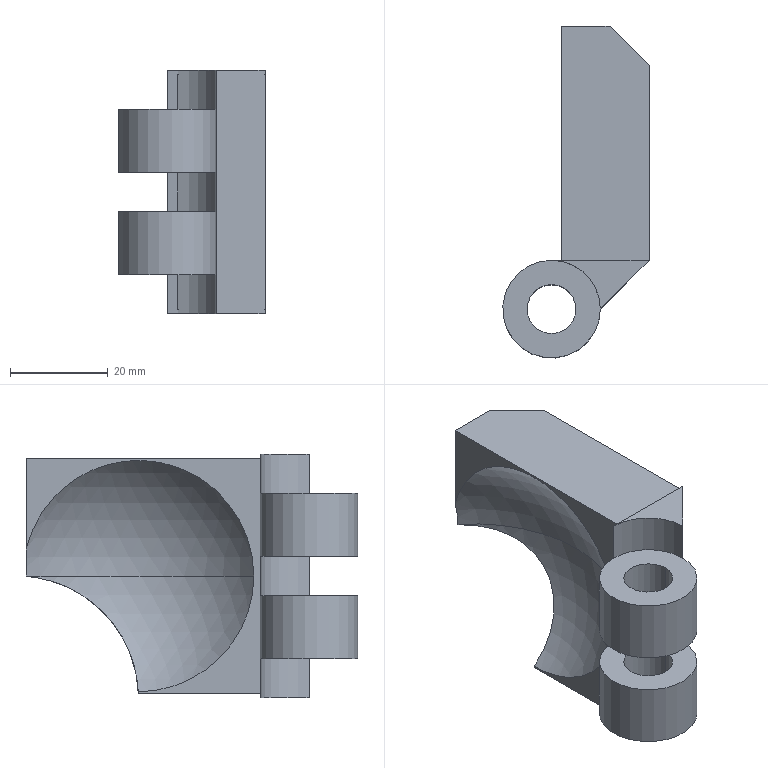Part | SolidWorks | features BaseBody 1 | 1 solid | 26 faces | box 30 x 68 x 50 mm | volume 32922 mm3 | plane 14 | cylinder 10 | sphere 2 | commonest cylinder face diameters 20 x5 10 x4 50 x1
STEP:
#1=CARTESIAN_POINT('',(-5.,0.,21.));
#2=VERTEX_POINT('',#1);
#3=CARTESIAN_POINT('',(5.,0.,21.));
#4=VERTEX_POINT('',#3);
#5=CARTESIAN_POINT('',(0.,0.,21.));
#6=DIRECTION('',(0.,0.,1.));
#7=DIRECTION('',(-1.,0.,0.));
#8=AXIS2_PLACEMENT_3D('',#5,#6,#7);
#9=CIRCLE('',#8,5.);
#10=EDGE_CURVE('',#2,#4,#9,.T.);
#11=ORIENTED_EDGE('',*,*,#10,.T.);
#12=CARTESIAN_POINT('',(5.,0.,8.));
#13=VERTEX_POINT('',#12);
#14=CARTESIAN_POINT('',(5.,0.,0.));
#15=DIRECTION('',(0.,0.,-1.));
#16=VECTOR('',#15,1000.);
#17=LINE('',#14,#16);
#18=EDGE_CURVE('',#4,#13,#17,.T.);
#19=ORIENTED_EDGE('',*,*,#18,.T.);
#20=CARTESIAN_POINT('',(-5.,0.,8.));
#21=VERTEX_POINT('',#20);
#22=CARTESIAN_POINT('',(0.,0.,8.));
#23=DIRECTION('',(0.,0.,-1.));
#24=DIRECTION('',(-1.,0.,0.));
#25=AXIS2_PLACEMENT_3D('',#22,#23,#24);
#26=CIRCLE('',#25,5.);
#27=EDGE_CURVE('',#13,#21,#26,.T.);
#28=ORIENTED_EDGE('',*,*,#27,.T.);
#29=CARTESIAN_POINT('',(-5.,0.,0.));
#30=DIRECTION('',(0.,0.,-1.));
#31=VECTOR('',#30,1000.);
#32=LINE('',#29,#31);
#33=EDGE_CURVE('',#2,#21,#32,.T.);
#34=ORIENTED_EDGE('',*,*,#33,.F.);
#35=EDGE_LOOP('',(#11,#19,#28,#34));
#36=FACE_OUTER_BOUND('',#35,.T.);
#37=CARTESIAN_POINT('',(0.,0.,0.));
#38=DIRECTION('',(0.,0.,-1.));
#39=DIRECTION('',(-1.,0.,0.));
#40=AXIS2_PLACEMENT_3D('',#37,#38,#39);
#41=CYLINDRICAL_SURFACE('',#40,5.);
#42=ADVANCED_FACE('',(#36),#41,.F.);
#43=CARTESIAN_POINT('',(2.,35.036,1.342));
#44=VERTEX_POINT('',#43);
#45=CARTESIAN_POINT('',(2.,11.342,25.));
#46=VERTEX_POINT('',#45);
#47=CARTESIAN_POINT('',(2.,35.,25.));
#48=DIRECTION('',(-1.,0.,0.));
#49=DIRECTION('',(0.,0.,1.));
#50=AXIS2_PLACEMENT_3D('',#47,#48,#49);
#51=CIRCLE('',#50,23.658);
#52=EDGE_CURVE('',#44,#46,#51,.T.);
#53=ORIENTED_EDGE('',*,*,#52,.T.);
#54=CARTESIAN_POINT('',(2.865,58.,25.));
#55=VERTEX_POINT('',#54);
#56=CARTESIAN_POINT('',(-15.321,35.,25.));
#57=DIRECTION('',(0.,0.,1.));
#58=DIRECTION('',(1.,0.,0.));
#59=AXIS2_PLACEMENT_3D('',#56,#57,#58);
#60=CIRCLE('',#59,29.321);
#61=EDGE_CURVE('',#46,#55,#60,.T.);
#62=ORIENTED_EDGE('',*,*,#61,.T.);
#63=CARTESIAN_POINT('',(2.865,58.,24.92));
#64=VERTEX_POINT('',#63);
#65=CARTESIAN_POINT('',(-15.321,58.,25.));
#66=DIRECTION('',(0.,1.,0.));
#67=DIRECTION('',(0.,0.,1.));
#68=AXIS2_PLACEMENT_3D('',#65,#66,#67);
#69=CIRCLE('',#68,18.186);
#70=EDGE_CURVE('',#55,#64,#69,.T.);
#71=ORIENTED_EDGE('',*,*,#70,.T.);
#72=CARTESIAN_POINT('',(2.865,58.,24.92));
#73=CARTESIAN_POINT('',(4.253,56.902,24.832));
#74=CARTESIAN_POINT('',(5.518,55.699,24.663));
#75=CARTESIAN_POINT('',(6.944,54.07,24.289));
#76=CARTESIAN_POINT('',(7.221,53.738,24.206));
#77=CARTESIAN_POINT('',(7.76,53.062,24.021));
#78=CARTESIAN_POINT('',(8.021,52.717,23.918));
#79=CARTESIAN_POINT('',(8.769,51.678,23.586));
#80=CARTESIAN_POINT('',(9.224,50.976,23.327));
#81=CARTESIAN_POINT('',(10.044,49.559,22.728));
#82=CARTESIAN_POINT('',(10.409,48.843,22.387));
#83=CARTESIAN_POINT('',(10.887,47.761,21.803));
#84=CARTESIAN_POINT('',(11.035,47.398,21.596));
#85=CARTESIAN_POINT('',(11.304,46.674,21.156));
#86=CARTESIAN_POINT('',(11.424,46.316,20.927));
#87=CARTESIAN_POINT('',(11.74,45.258,20.209));
#88=CARTESIAN_POINT('',(11.894,44.572,19.691));
#89=CARTESIAN_POINT('',(12.039,43.575,18.852));
#90=CARTESIAN_POINT('',(12.073,43.248,18.562));
#91=CARTESIAN_POINT('',(12.111,42.604,17.96));
#92=CARTESIAN_POINT('',(12.116,42.286,17.647));
#93=CARTESIAN_POINT('',(12.082,41.364,16.688));
#94=CARTESIAN_POINT('',(11.999,40.792,16.025));
#95=CARTESIAN_POINT('',(11.789,39.994,14.998));
#96=CARTESIAN_POINT('',(11.704,39.738,14.65));
#97=CARTESIAN_POINT('',(11.506,39.246,13.944));
#98=CARTESIAN_POINT('',(11.391,39.008,13.584));
#99=CARTESIAN_POINT('',(11.008,38.334,12.502));
#100=CARTESIAN_POINT('',(10.7,37.935,11.78));
#101=CARTESIAN_POINT('',(10.166,37.401,10.697));
#102=CARTESIAN_POINT('',(9.975,37.234,10.336));
#103=CARTESIAN_POINT('',(9.57,36.92,9.616));
#104=CARTESIAN_POINT('',(9.354,36.773,9.255));
#105=CARTESIAN_POINT('',(8.225,36.094,7.472));
#106=CARTESIAN_POINT('',(7.167,35.724,6.114));
#107=CARTESIAN_POINT('',(4.755,35.22,3.557));
#108=CARTESIAN_POINT('',(3.432,35.092,2.39));
#109=CARTESIAN_POINT('',(2.,35.036,1.342));
#110=B_SPLINE_CURVE_WITH_KNOTS('',3,(#72,#73,#74,#75,#76,#77,#78,#79,#80,#81,#82,#83,#84,#85,#86,#87,#88,#89,#90,#91,#92,#93,#94,#95,#96,#97,#98,#99,#100,#101,#102,#103,#104,#105,#106,#107,#108,#109),.UNSPECIFIED.,.F.,.F.,(4,2,2,2,2,2,2,2,2,2,2,2,2,2,2,2,2,2,4),(0.,0.005258,0.006573,0.007887,0.01052,0.01315,0.01446,0.01577,0.0184,0.01972,0.02103,0.02366,0.02498,0.02629,0.02892,0.03023,0.03155,0.03681,0.04206),.UNSPECIFIED.);
#111=EDGE_CURVE('',#64,#44,#110,.T.);
#112=ORIENTED_EDGE('',*,*,#111,.T.);
#113=EDGE_LOOP('',(#53,#62,#71,#112));
#114=FACE_OUTER_BOUND('',#113,.T.);
#115=CARTESIAN_POINT('',(-15.321,35.,25.));
#116=DIRECTION('',(0.,0.,-1.));
#117=DIRECTION('',(1.,0.,0.));
#118=AXIS2_PLACEMENT_3D('',#115,#116,#117);
#119=SPHERICAL_SURFACE('',#118,29.321);
#120=ADVANCED_FACE('',(#114),#119,.F.);
#121=CARTESIAN_POINT('',(-5.,0.,42.));
#122=VERTEX_POINT('',#121);
#123=CARTESIAN_POINT('',(5.,0.,42.));
#124=VERTEX_POINT('',#123);
#125=CARTESIAN_POINT('',(0.,0.,42.));
#126=DIRECTION('',(0.,0.,1.));
#127=DIRECTION('',(-1.,0.,0.));
#128=AXIS2_PLACEMENT_3D('',#125,#126,#127);
#129=CIRCLE('',#128,5.);
#130=EDGE_CURVE('',#122,#124,#129,.T.);
#131=ORIENTED_EDGE('',*,*,#130,.T.);
#132=CARTESIAN_POINT('',(5.,0.,29.));
#133=VERTEX_POINT('',#132);
#134=CARTESIAN_POINT('',(5.,0.,0.));
#135=DIRECTION('',(0.,0.,-1.));
#136=VECTOR('',#135,1000.);
#137=LINE('',#134,#136);
#138=EDGE_CURVE('',#124,#133,#137,.T.);
#139=ORIENTED_EDGE('',*,*,#138,.T.);
#140=CARTESIAN_POINT('',(-5.,0.,29.));
#141=VERTEX_POINT('',#140);
#142=CARTESIAN_POINT('',(0.,0.,29.));
#143=DIRECTION('',(0.,0.,-1.));
#144=DIRECTION('',(-1.,0.,0.));
#145=AXIS2_PLACEMENT_3D('',#142,#143,#144);
#146=CIRCLE('',#145,5.);
#147=EDGE_CURVE('',#133,#141,#146,.T.);
#148=ORIENTED_EDGE('',*,*,#147,.T.);
#149=CARTESIAN_POINT('',(-5.,0.,0.));
#150=DIRECTION('',(0.,0.,-1.));
#151=VECTOR('',#150,1000.);
#152=LINE('',#149,#151);
#153=EDGE_CURVE('',#122,#141,#152,.T.);
#154=ORIENTED_EDGE('',*,*,#153,.F.);
#155=EDGE_LOOP('',(#131,#139,#148,#154));
#156=FACE_OUTER_BOUND('',#155,.T.);
#157=CARTESIAN_POINT('',(0.,0.,0.));
#158=DIRECTION('',(0.,0.,-1.));
#159=DIRECTION('',(-1.,0.,0.));
#160=AXIS2_PLACEMENT_3D('',#157,#158,#159);
#161=CYLINDRICAL_SURFACE('',#160,5.);
#162=ADVANCED_FACE('',(#156),#161,.F.);
#163=CARTESIAN_POINT('',(0.,0.,29.));
#164=DIRECTION('',(0.,0.,-1.));
#165=DIRECTION('',(-1.,0.,0.));
#166=AXIS2_PLACEMENT_3D('',#163,#164,#165);
#167=CIRCLE('',#166,5.);
#168=EDGE_CURVE('',#141,#133,#167,.T.);
#169=ORIENTED_EDGE('',*,*,#168,.F.);
#170=ORIENTED_EDGE('',*,*,#147,.F.);
#171=EDGE_LOOP('',(#169,#170));
#172=FACE_BOUND('',#171,.T.);
#173=CARTESIAN_POINT('',(0.,10.,29.));
#174=VERTEX_POINT('',#173);
#175=CARTESIAN_POINT('',(10.,0.,29.));
#176=VERTEX_POINT('',#175);
#177=CARTESIAN_POINT('',(0.,0.,29.));
#178=DIRECTION('',(0.,0.,1.));
#179=DIRECTION('',(0.,1.,0.));
#180=AXIS2_PLACEMENT_3D('',#177,#178,#179);
#181=CIRCLE('',#180,10.);
#182=EDGE_CURVE('',#174,#176,#181,.T.);
#183=ORIENTED_EDGE('',*,*,#182,.F.);
#184=CARTESIAN_POINT('',(0.,0.,29.));
#185=DIRECTION('',(0.,0.,-1.));
#186=DIRECTION('',(1.,0.,0.));
#187=AXIS2_PLACEMENT_3D('',#184,#185,#186);
#188=CIRCLE('',#187,10.);
#189=EDGE_CURVE('',#174,#176,#188,.T.);
#190=ORIENTED_EDGE('',*,*,#189,.T.);
#191=EDGE_LOOP('',(#183,#190));
#192=FACE_OUTER_BOUND('',#191,.T.);
#193=CARTESIAN_POINT('',(-10.,0.,29.));
#194=DIRECTION('',(0.,0.,1.));
#195=DIRECTION('',(1.,0.,0.));
#196=AXIS2_PLACEMENT_3D('',#193,#194,#195);
#197=PLANE('',#196);
#198=ADVANCED_FACE('',(#172,#192),#197,.F.);
#199=CARTESIAN_POINT('',(10.,0.,21.));
#200=VERTEX_POINT('',#199);
#201=CARTESIAN_POINT('',(10.,0.,0.));
#202=DIRECTION('',(0.,0.,1.));
#203=VECTOR('',#202,1000.);
#204=LINE('',#201,#203);
#205=EDGE_CURVE('',#200,#176,#204,.T.);
#206=ORIENTED_EDGE('',*,*,#205,.T.);
#207=ORIENTED_EDGE('',*,*,#189,.F.);
#208=CARTESIAN_POINT('',(0.,10.,21.));
#209=VERTEX_POINT('',#208);
#210=CARTESIAN_POINT('',(0.,10.,0.));
#211=DIRECTION('',(0.,0.,1.));
#212=VECTOR('',#211,1000.);
#213=LINE('',#210,#212);
#214=EDGE_CURVE('',#209,#174,#213,.T.);
#215=ORIENTED_EDGE('',*,*,#214,.F.);
#216=CARTESIAN_POINT('',(0.,0.,21.));
#217=DIRECTION('',(0.,0.,-1.));
#218=DIRECTION('',(1.,0.,0.));
#219=AXIS2_PLACEMENT_3D('',#216,#217,#218);
#220=CIRCLE('',#219,10.);
#221=EDGE_CURVE('',#209,#200,#220,.T.);
#222=ORIENTED_EDGE('',*,*,#221,.T.);
#223=EDGE_LOOP('',(#206,#207,#215,#222));
#224=FACE_OUTER_BOUND('',#223,.T.);
#225=CARTESIAN_POINT('',(0.,0.,25.));
#226=DIRECTION('',(0.,0.,1.));
#227=DIRECTION('',(-1.,0.,0.));
#228=AXIS2_PLACEMENT_3D('',#225,#226,#227);
#229=CYLINDRICAL_SURFACE('',#228,10.);
#230=ADVANCED_FACE('',(#224),#229,.F.);
#231=ORIENTED_EDGE('',*,*,#10,.F.);
#232=CARTESIAN_POINT('',(0.,0.,21.));
#233=DIRECTION('',(0.,0.,1.));
#234=DIRECTION('',(-1.,0.,0.));
#235=AXIS2_PLACEMENT_3D('',#232,#233,#234);
#236=CIRCLE('',#235,5.);
#237=EDGE_CURVE('',#4,#2,#236,.T.);
#238=ORIENTED_EDGE('',*,*,#237,.F.);
#239=EDGE_LOOP('',(#231,#238));
#240=FACE_BOUND('',#239,.T.);
#241=CARTESIAN_POINT('',(0.,0.,21.));
#242=DIRECTION('',(0.,0.,-1.));
#243=DIRECTION('',(0.,1.,0.));
#244=AXIS2_PLACEMENT_3D('',#241,#242,#243);
#245=CIRCLE('',#244,10.);
#246=EDGE_CURVE('',#200,#209,#245,.T.);
#247=ORIENTED_EDGE('',*,*,#246,.F.);
#248=ORIENTED_EDGE('',*,*,#221,.F.);
#249=EDGE_LOOP('',(#247,#248));
#250=FACE_OUTER_BOUND('',#249,.T.);
#251=CARTESIAN_POINT('',(0.,0.,21.));
#252=DIRECTION('',(0.,0.,-1.));
#253=DIRECTION('',(0.,-1.,0.));
#254=AXIS2_PLACEMENT_3D('',#251,#252,#253);
#255=PLANE('',#254);
#256=ADVANCED_FACE('',(#240,#250),#255,.F.);
#257=CARTESIAN_POINT('',(0.,0.,8.));
#258=DIRECTION('',(0.,0.,-1.));
#259=DIRECTION('',(-1.,0.,0.));
#260=AXIS2_PLACEMENT_3D('',#257,#258,#259);
#261=CIRCLE('',#260,5.);
#262=EDGE_CURVE('',#21,#13,#261,.T.);
#263=ORIENTED_EDGE('',*,*,#262,.F.);
#264=ORIENTED_EDGE('',*,*,#27,.F.);
#265=EDGE_LOOP('',(#263,#264));
#266=FACE_BOUND('',#265,.T.);
#267=CARTESIAN_POINT('',(0.,10.,8.));
#268=VERTEX_POINT('',#267);
#269=CARTESIAN_POINT('',(10.,0.,8.));
#270=VERTEX_POINT('',#269);
#271=CARTESIAN_POINT('',(0.,0.,8.));
#272=DIRECTION('',(0.,0.,1.));
#273=DIRECTION('',(0.,1.,0.));
#274=AXIS2_PLACEMENT_3D('',#271,#272,#273);
#275=CIRCLE('',#274,10.);
#276=EDGE_CURVE('',#268,#270,#275,.T.);
#277=ORIENTED_EDGE('',*,*,#276,.F.);
#278=CARTESIAN_POINT('',(0.,0.,8.));
#279=DIRECTION('',(0.,0.,-1.));
#280=DIRECTION('',(1.,0.,0.));
#281=AXIS2_PLACEMENT_3D('',#278,#279,#280);
#282=CIRCLE('',#281,10.);
#283=EDGE_CURVE('',#268,#270,#282,.T.);
#284=ORIENTED_EDGE('',*,*,#283,.T.);
#285=EDGE_LOOP('',(#277,#284));
#286=FACE_OUTER_BOUND('',#285,.T.);
#287=CARTESIAN_POINT('',(-10.,0.,8.));
#288=DIRECTION('',(0.,0.,1.));
#289=DIRECTION('',(1.,0.,0.));
#290=AXIS2_PLACEMENT_3D('',#287,#288,#289);
#291=PLANE('',#290);
#292=ADVANCED_FACE('',(#266,#286),#291,.F.);
#293=CARTESIAN_POINT('',(10.,0.,0.));
#294=VERTEX_POINT('',#293);
#295=CARTESIAN_POINT('',(10.,0.,0.));
#296=DIRECTION('',(0.,0.,1.));
#297=VECTOR('',#296,1000.);
#298=LINE('',#295,#297);
#299=EDGE_CURVE('',#294,#270,#298,.T.);
#300=ORIENTED_EDGE('',*,*,#299,.T.);
#301=ORIENTED_EDGE('',*,*,#283,.F.);
#302=CARTESIAN_POINT('',(0.,10.,0.));
#303=VERTEX_POINT('',#302);
#304=CARTESIAN_POINT('',(0.,10.,0.));
#305=DIRECTION('',(0.,0.,1.));
#306=VECTOR('',#305,1000.);
#307=LINE('',#304,#306);
#308=EDGE_CURVE('',#303,#268,#307,.T.);
#309=ORIENTED_EDGE('',*,*,#308,.F.);
#310=CARTESIAN_POINT('',(0.,0.,0.));
#311=DIRECTION('',(0.,0.,1.));
#312=DIRECTION('',(-1.,0.,0.));
#313=AXIS2_PLACEMENT_3D('',#310,#311,#312);
#314=CIRCLE('',#313,10.);
#315=EDGE_CURVE('',#294,#303,#314,.T.);
#316=ORIENTED_EDGE('',*,*,#315,.F.);
#317=EDGE_LOOP('',(#300,#301,#309,#316));
#318=FACE_OUTER_BOUND('',#317,.T.);
#319=CARTESIAN_POINT('',(0.,0.,4.));
#320=DIRECTION('',(0.,0.,1.));
#321=DIRECTION('',(-1.,0.,0.));
#322=AXIS2_PLACEMENT_3D('',#319,#320,#321);
#323=CYLINDRICAL_SURFACE('',#322,10.);
#324=ADVANCED_FACE('',(#318),#323,.F.);
#325=CARTESIAN_POINT('',(10.,0.,42.));
#326=VERTEX_POINT('',#325);
#327=CARTESIAN_POINT('',(10.,0.,50.));
#328=VERTEX_POINT('',#327);
#329=CARTESIAN_POINT('',(10.,0.,0.));
#330=DIRECTION('',(0.,0.,1.));
#331=VECTOR('',#330,1000.);
#332=LINE('',#329,#331);
#333=EDGE_CURVE('',#326,#328,#332,.T.);
#334=ORIENTED_EDGE('',*,*,#333,.T.);
#335=CARTESIAN_POINT('',(0.,10.,50.));
#336=VERTEX_POINT('',#335);
#337=CARTESIAN_POINT('',(0.,0.,50.));
#338=DIRECTION('',(0.,0.,-1.));
#339=DIRECTION('',(-1.,0.,0.));
#340=AXIS2_PLACEMENT_3D('',#337,#338,#339);
#341=CIRCLE('',#340,10.);
#342=EDGE_CURVE('',#336,#328,#341,.T.);
#343=ORIENTED_EDGE('',*,*,#342,.F.);
#344=CARTESIAN_POINT('',(0.,10.,42.));
#345=VERTEX_POINT('',#344);
#346=CARTESIAN_POINT('',(0.,10.,0.));
#347=DIRECTION('',(0.,0.,1.));
#348=VECTOR('',#347,1000.);
#349=LINE('',#346,#348);
#350=EDGE_CURVE('',#345,#336,#349,.T.);
#351=ORIENTED_EDGE('',*,*,#350,.F.);
#352=CARTESIAN_POINT('',(0.,0.,42.));
#353=DIRECTION('',(0.,0.,-1.));
#354=DIRECTION('',(1.,0.,0.));
#355=AXIS2_PLACEMENT_3D('',#352,#353,#354);
#356=CIRCLE('',#355,10.);
#357=EDGE_CURVE('',#345,#326,#356,.T.);
#358=ORIENTED_EDGE('',*,*,#357,.T.);
#359=EDGE_LOOP('',(#334,#343,#351,#358));
#360=FACE_OUTER_BOUND('',#359,.T.);
#361=CARTESIAN_POINT('',(0.,0.,46.));
#362=DIRECTION('',(0.,0.,1.));
#363=DIRECTION('',(-1.,0.,0.));
#364=AXIS2_PLACEMENT_3D('',#361,#362,#363);
#365=CYLINDRICAL_SURFACE('',#364,10.);
#366=ADVANCED_FACE('',(#360),#365,.F.);
#367=ORIENTED_EDGE('',*,*,#130,.F.);
#368=CARTESIAN_POINT('',(0.,0.,42.));
#369=DIRECTION('',(0.,0.,1.));
#370=DIRECTION('',(-1.,0.,0.));
#371=AXIS2_PLACEMENT_3D('',#368,#369,#370);
#372=CIRCLE('',#371,5.);
#373=EDGE_CURVE('',#124,#122,#372,.T.);
#374=ORIENTED_EDGE('',*,*,#373,.F.);
#375=EDGE_LOOP('',(#367,#374));
#376=FACE_BOUND('',#375,.T.);
#377=CARTESIAN_POINT('',(0.,0.,42.));
#378=DIRECTION('',(0.,0.,-1.));
#379=DIRECTION('',(0.,1.,0.));
#380=AXIS2_PLACEMENT_3D('',#377,#378,#379);
#381=CIRCLE('',#380,10.);
#382=EDGE_CURVE('',#326,#345,#381,.T.);
#383=ORIENTED_EDGE('',*,*,#382,.F.);
#384=ORIENTED_EDGE('',*,*,#357,.F.);
#385=EDGE_LOOP('',(#383,#384));
#386=FACE_OUTER_BOUND('',#385,.T.);
#387=CARTESIAN_POINT('',(0.,0.,42.));
#388=DIRECTION('',(0.,0.,-1.));
#389=DIRECTION('',(0.,-1.,0.));
#390=AXIS2_PLACEMENT_3D('',#387,#388,#389);
#391=PLANE('',#390);
#392=ADVANCED_FACE('',(#376,#386),#391,.F.);
#393=ORIENTED_EDGE('',*,*,#315,.T.);
#394=CARTESIAN_POINT('',(20.,10.,0.));
#395=VERTEX_POINT('',#394);
#396=CARTESIAN_POINT('',(7.926,10.,0.));
#397=DIRECTION('',(1.,0.,0.));
#398=VECTOR('',#397,1000.);
#399=LINE('',#396,#398);
#400=EDGE_CURVE('',#303,#395,#399,.T.);
#401=ORIENTED_EDGE('',*,*,#400,.T.);
#402=CARTESIAN_POINT('',(10.,0.,0.));
#403=DIRECTION('',(0.7071,0.7071,0.));
#404=VECTOR('',#403,1000.);
#405=LINE('',#402,#404);
#406=EDGE_CURVE('',#294,#395,#405,.T.);
#407=ORIENTED_EDGE('',*,*,#406,.F.);
#408=EDGE_LOOP('',(#393,#401,#407));
#409=FACE_OUTER_BOUND('',#408,.T.);
#410=CARTESIAN_POINT('',(4.852,2.817,0.));
#411=DIRECTION('',(0.,0.,1.));
#412=DIRECTION('',(1.,0.,0.));
#413=AXIS2_PLACEMENT_3D('',#410,#411,#412);
#414=PLANE('',#413);
#415=ADVANCED_FACE('',(#409),#414,.F.);
#416=ORIENTED_EDGE('',*,*,#182,.T.);
#417=CARTESIAN_POINT('',(10.,0.,0.));
#418=DIRECTION('',(0.,0.,1.));
#419=VECTOR('',#418,1000.);
#420=LINE('',#417,#419);
#421=EDGE_CURVE('',#176,#326,#420,.T.);
#422=ORIENTED_EDGE('',*,*,#421,.T.);
#423=ORIENTED_EDGE('',*,*,#382,.T.);
#424=CARTESIAN_POINT('',(0.,10.,0.));
#425=DIRECTION('',(0.,0.,1.));
#426=VECTOR('',#425,1000.);
#427=LINE('',#424,#426);
#428=EDGE_CURVE('',#174,#345,#427,.T.);
#429=ORIENTED_EDGE('',*,*,#428,.F.);
#430=EDGE_LOOP('',(#416,#422,#423,#429));
#431=FACE_OUTER_BOUND('',#430,.T.);
#432=CARTESIAN_POINT('',(0.,0.,0.));
#433=DIRECTION('',(0.,0.,-1.));
#434=DIRECTION('',(0.,1.,0.));
#435=AXIS2_PLACEMENT_3D('',#432,#433,#434);
#436=CYLINDRICAL_SURFACE('',#435,10.);
#437=ADVANCED_FACE('',(#431),#436,.T.);
#438=ORIENTED_EDGE('',*,*,#246,.T.);
#439=CARTESIAN_POINT('',(0.,10.,0.));
#440=DIRECTION('',(0.,0.,1.));
#441=VECTOR('',#440,1000.);
#442=LINE('',#439,#441);
#443=EDGE_CURVE('',#268,#209,#442,.T.);
#444=ORIENTED_EDGE('',*,*,#443,.F.);
#445=ORIENTED_EDGE('',*,*,#276,.T.);
#446=CARTESIAN_POINT('',(10.,0.,0.));
#447=DIRECTION('',(0.,0.,1.));
#448=VECTOR('',#447,1000.);
#449=LINE('',#446,#448);
#450=EDGE_CURVE('',#270,#200,#449,.T.);
#451=ORIENTED_EDGE('',*,*,#450,.T.);
#452=EDGE_LOOP('',(#438,#444,#445,#451));
#453=FACE_OUTER_BOUND('',#452,.T.);
#454=CARTESIAN_POINT('',(0.,0.,0.));
#455=DIRECTION('',(0.,0.,-1.));
#456=DIRECTION('',(0.,1.,0.));
#457=AXIS2_PLACEMENT_3D('',#454,#455,#456);
#458=CYLINDRICAL_SURFACE('',#457,10.);
#459=ADVANCED_FACE('',(#453),#458,.T.);
#460=ORIENTED_EDGE('',*,*,#111,.F.);
#461=CARTESIAN_POINT('',(12.,58.,24.92));
#462=VERTEX_POINT('',#461);
#463=CARTESIAN_POINT('',(2.,58.,24.92));
#464=DIRECTION('',(-1.,0.,0.));
#465=VECTOR('',#464,1000.);
#466=LINE('',#463,#465);
#467=EDGE_CURVE('',#462,#64,#466,.T.);
#468=ORIENTED_EDGE('',*,*,#467,.F.);
#469=CARTESIAN_POINT('',(20.,50.,22.913));
#470=VERTEX_POINT('',#469);
#471=CARTESIAN_POINT('',(20.,50.,22.913));
#472=CARTESIAN_POINT('',(17.457,52.543,24.023));
#473=CARTESIAN_POINT('',(14.766,55.234,24.698));
#474=CARTESIAN_POINT('',(12.,58.,24.92));
#475=(BOUNDED_CURVE()B_SPLINE_CURVE(3,(#471,#472,#473,#474),.UNSPECIFIED.,.F.,.F.)B_SPLINE_CURVE_WITH_KNOTS((4,4),(4.301,4.632),.UNSPECIFIED.)CURVE()GEOMETRIC_REPRESENTATION_ITEM()RATIONAL_B_SPLINE_CURVE((1.,0.9909,0.9909,1.))REPRESENTATION_ITEM(''));
#476=EDGE_CURVE('',#470,#462,#475,.T.);
#477=ORIENTED_EDGE('',*,*,#476,.F.);
#478=CARTESIAN_POINT('',(20.,35.02,1.));
#479=VERTEX_POINT('',#478);
#480=CARTESIAN_POINT('',(20.,60.,0.));
#481=DIRECTION('',(-1.,0.,0.));
#482=DIRECTION('',(0.,0.,-1.));
#483=AXIS2_PLACEMENT_3D('',#480,#481,#482);
#484=CIRCLE('',#483,25.);
#485=EDGE_CURVE('',#479,#470,#484,.T.);
#486=ORIENTED_EDGE('',*,*,#485,.F.);
#487=CARTESIAN_POINT('',(2.,35.02,1.));
#488=VERTEX_POINT('',#487);
#489=CARTESIAN_POINT('',(2.,35.02,1.));
#490=DIRECTION('',(1.,0.,0.));
#491=VECTOR('',#490,1000.);
#492=LINE('',#489,#491);
#493=EDGE_CURVE('',#488,#479,#492,.T.);
#494=ORIENTED_EDGE('',*,*,#493,.F.);
#495=CARTESIAN_POINT('',(2.,60.,0.));
#496=DIRECTION('',(1.,0.,0.));
#497=DIRECTION('',(0.,0.,-1.));
#498=AXIS2_PLACEMENT_3D('',#495,#496,#497);
#499=CIRCLE('',#498,25.);
#500=EDGE_CURVE('',#44,#488,#499,.T.);
#501=ORIENTED_EDGE('',*,*,#500,.F.);
#502=EDGE_LOOP('',(#460,#468,#477,#486,#494,#501));
#503=FACE_OUTER_BOUND('',#502,.T.);
#504=CARTESIAN_POINT('',(2.,60.,0.));
#505=DIRECTION('',(-1.,0.,0.));
#506=DIRECTION('',(0.,0.,-1.));
#507=AXIS2_PLACEMENT_3D('',#504,#505,#506);
#508=CYLINDRICAL_SURFACE('',#507,25.);
#509=ADVANCED_FACE('',(#503),#508,.F.);
#510=ORIENTED_EDGE('',*,*,#467,.T.);
#511=ORIENTED_EDGE('',*,*,#70,.F.);
#512=CARTESIAN_POINT('',(2.,58.,30.542));
#513=VERTEX_POINT('',#512);
#514=CARTESIAN_POINT('',(-15.321,58.,25.));
#515=DIRECTION('',(0.,1.,0.));
#516=DIRECTION('',(0.,0.,1.));
#517=AXIS2_PLACEMENT_3D('',#514,#515,#516);
#518=CIRCLE('',#517,18.186);
#519=EDGE_CURVE('',#513,#55,#518,.T.);
#520=ORIENTED_EDGE('',*,*,#519,.F.);
#521=CARTESIAN_POINT('',(2.,58.,49.));
#522=VERTEX_POINT('',#521);
#523=CARTESIAN_POINT('',(2.,58.,50.));
#524=DIRECTION('',(0.,0.,-1.));
#525=VECTOR('',#524,1000.);
#526=LINE('',#523,#525);
#527=EDGE_CURVE('',#522,#513,#526,.T.);
#528=ORIENTED_EDGE('',*,*,#527,.F.);
#529=CARTESIAN_POINT('',(12.,58.,49.));
#530=VERTEX_POINT('',#529);
#531=CARTESIAN_POINT('',(7.,58.,49.));
#532=DIRECTION('',(1.,0.,0.));
#533=VECTOR('',#532,1000.);
#534=LINE('',#531,#533);
#535=EDGE_CURVE('',#522,#530,#534,.T.);
#536=ORIENTED_EDGE('',*,*,#535,.T.);
#537=CARTESIAN_POINT('',(12.,58.,25.));
#538=DIRECTION('',(0.,0.,1.));
#539=VECTOR('',#538,1000.);
#540=LINE('',#537,#539);
#541=EDGE_CURVE('',#462,#530,#540,.T.);
#542=ORIENTED_EDGE('',*,*,#541,.F.);
#543=EDGE_LOOP('',(#510,#511,#520,#528,#536,#542));
#544=FACE_OUTER_BOUND('',#543,.T.);
#545=CARTESIAN_POINT('',(12.,58.,50.));
#546=DIRECTION('',(0.,-1.,0.));
#547=DIRECTION('',(0.,0.,-1.));
#548=AXIS2_PLACEMENT_3D('',#545,#546,#547);
#549=PLANE('',#548);
#550=ADVANCED_FACE('',(#544),#549,.F.);
#551=ORIENTED_EDGE('',*,*,#500,.T.);
#552=CARTESIAN_POINT('',(2.,10.,1.));
#553=VERTEX_POINT('',#552);
#554=CARTESIAN_POINT('',(2.,59.,1.));
#555=DIRECTION('',(0.,-1.,0.));
#556=VECTOR('',#555,1000.);
#557=LINE('',#554,#556);
#558=EDGE_CURVE('',#488,#553,#557,.T.);
#559=ORIENTED_EDGE('',*,*,#558,.T.);
#560=CARTESIAN_POINT('',(2.,10.,49.));
#561=VERTEX_POINT('',#560);
#562=CARTESIAN_POINT('',(2.,10.,50.));
#563=DIRECTION('',(0.,0.,-1.));
#564=VECTOR('',#563,1000.);
#565=LINE('',#562,#564);
#566=EDGE_CURVE('',#561,#553,#565,.T.);
#567=ORIENTED_EDGE('',*,*,#566,.F.);
#568=CARTESIAN_POINT('',(2.,59.,49.));
#569=DIRECTION('',(0.,1.,0.));
#570=VECTOR('',#569,1000.);
#571=LINE('',#568,#570);
#572=EDGE_CURVE('',#561,#522,#571,.T.);
#573=ORIENTED_EDGE('',*,*,#572,.T.);
#574=ORIENTED_EDGE('',*,*,#527,.T.);
#575=CARTESIAN_POINT('',(2.,35.,25.));
#576=DIRECTION('',(-1.,0.,0.));
#577=DIRECTION('',(0.,0.,1.));
#578=AXIS2_PLACEMENT_3D('',#575,#576,#577);
#579=CIRCLE('',#578,23.658);
#580=EDGE_CURVE('',#46,#513,#579,.T.);
#581=ORIENTED_EDGE('',*,*,#580,.F.);
#582=ORIENTED_EDGE('',*,*,#52,.F.);
#583=EDGE_LOOP('',(#551,#559,#567,#573,#574,#581,#582));
#584=FACE_OUTER_BOUND('',#583,.T.);
#585=CARTESIAN_POINT('',(2.,60.,50.));
#586=DIRECTION('',(1.,0.,0.));
#587=DIRECTION('',(0.,1.,0.));
#588=AXIS2_PLACEMENT_3D('',#585,#586,#587);
#589=PLANE('',#588);
#590=ADVANCED_FACE('',(#584),#589,.F.);
#591=ORIENTED_EDGE('',*,*,#493,.T.);
#592=CARTESIAN_POINT('',(20.,10.,1.));
#593=VERTEX_POINT('',#592);
#594=CARTESIAN_POINT('',(20.,34.,1.));
#595=DIRECTION('',(0.,1.,0.));
#596=VECTOR('',#595,1000.);
#597=LINE('',#594,#596);
#598=EDGE_CURVE('',#593,#479,#597,.T.);
#599=ORIENTED_EDGE('',*,*,#598,.F.);
#600=CARTESIAN_POINT('',(2.,10.,1.));
#601=DIRECTION('',(-1.,0.,0.));
#602=VECTOR('',#601,1000.);
#603=LINE('',#600,#602);
#604=EDGE_CURVE('',#593,#553,#603,.T.);
#605=ORIENTED_EDGE('',*,*,#604,.T.);
#606=ORIENTED_EDGE('',*,*,#558,.F.);
#607=EDGE_LOOP('',(#591,#599,#605,#606));
#608=FACE_OUTER_BOUND('',#607,.T.);
#609=CARTESIAN_POINT('',(20.,58.,1.));
#610=DIRECTION('',(0.,0.,1.));
#611=DIRECTION('',(1.,0.,0.));
#612=AXIS2_PLACEMENT_3D('',#609,#610,#611);
#613=PLANE('',#612);
#614=ADVANCED_FACE('',(#608),#613,.F.);
#615=CARTESIAN_POINT('',(20.,50.,49.));
#616=VERTEX_POINT('',#615);
#617=CARTESIAN_POINT('',(13.5,56.5,49.));
#618=DIRECTION('',(0.7071,-0.7071,0.));
#619=VECTOR('',#618,1000.);
#620=LINE('',#617,#619);
#621=EDGE_CURVE('',#530,#616,#620,.T.);
#622=ORIENTED_EDGE('',*,*,#621,.F.);
#623=ORIENTED_EDGE('',*,*,#535,.F.);
#624=ORIENTED_EDGE('',*,*,#572,.F.);
#625=CARTESIAN_POINT('',(20.,10.,49.));
#626=VERTEX_POINT('',#625);
#627=CARTESIAN_POINT('',(20.,10.,49.));
#628=DIRECTION('',(1.,0.,0.));
#629=VECTOR('',#628,1000.);
#630=LINE('',#627,#629);
#631=EDGE_CURVE('',#561,#626,#630,.T.);
#632=ORIENTED_EDGE('',*,*,#631,.T.);
#633=CARTESIAN_POINT('',(20.,34.,49.));
#634=DIRECTION('',(0.,-1.,0.));
#635=VECTOR('',#634,1000.);
#636=LINE('',#633,#635);
#637=EDGE_CURVE('',#616,#626,#636,.T.);
#638=ORIENTED_EDGE('',*,*,#637,.F.);
#639=EDGE_LOOP('',(#622,#623,#624,#632,#638));
#640=FACE_OUTER_BOUND('',#639,.T.);
#641=CARTESIAN_POINT('',(2.,58.,49.));
#642=DIRECTION('',(0.,0.,-1.));
#643=DIRECTION('',(-1.,0.,0.));
#644=AXIS2_PLACEMENT_3D('',#641,#642,#643);
#645=PLANE('',#644);
#646=ADVANCED_FACE('',(#640),#645,.F.);
#647=ORIENTED_EDGE('',*,*,#342,.T.);
#648=CARTESIAN_POINT('',(20.,10.,50.));
#649=VERTEX_POINT('',#648);
#650=CARTESIAN_POINT('',(10.,0.,50.));
#651=DIRECTION('',(0.7071,0.7071,0.));
#652=VECTOR('',#651,1000.);
#653=LINE('',#650,#652);
#654=EDGE_CURVE('',#328,#649,#653,.T.);
#655=ORIENTED_EDGE('',*,*,#654,.T.);
#656=CARTESIAN_POINT('',(7.926,10.,50.));
#657=DIRECTION('',(-1.,0.,0.));
#658=VECTOR('',#657,1000.);
#659=LINE('',#656,#658);
#660=EDGE_CURVE('',#649,#336,#659,.T.);
#661=ORIENTED_EDGE('',*,*,#660,.T.);
#662=EDGE_LOOP('',(#647,#655,#661));
#663=FACE_OUTER_BOUND('',#662,.T.);
#664=CARTESIAN_POINT('',(4.852,2.817,50.));
#665=DIRECTION('',(0.,0.,1.));
#666=DIRECTION('',(1.,0.,0.));
#667=AXIS2_PLACEMENT_3D('',#664,#665,#666);
#668=PLANE('',#667);
#669=ADVANCED_FACE('',(#663),#668,.T.);
#670=ORIENTED_EDGE('',*,*,#485,.T.);
#671=CARTESIAN_POINT('',(20.,50.,0.));
#672=DIRECTION('',(0.,0.,1.));
#673=VECTOR('',#672,1000.);
#674=LINE('',#671,#673);
#675=EDGE_CURVE('',#470,#616,#674,.T.);
#676=ORIENTED_EDGE('',*,*,#675,.T.);
#677=ORIENTED_EDGE('',*,*,#637,.T.);
#678=CARTESIAN_POINT('',(20.,10.,0.));
#679=DIRECTION('',(0.,0.,1.));
#680=VECTOR('',#679,1000.);
#681=LINE('',#678,#680);
#682=EDGE_CURVE('',#593,#626,#681,.T.);
#683=ORIENTED_EDGE('',*,*,#682,.F.);
#684=ORIENTED_EDGE('',*,*,#598,.T.);
#685=EDGE_LOOP('',(#670,#676,#677,#683,#684));
#686=FACE_OUTER_BOUND('',#685,.T.);
#687=CARTESIAN_POINT('',(20.,10.,0.));
#688=DIRECTION('',(1.,0.,0.));
#689=DIRECTION('',(0.,1.,0.));
#690=AXIS2_PLACEMENT_3D('',#687,#688,#689);
#691=PLANE('',#690);
#692=ADVANCED_FACE('',(#686),#691,.T.);
#693=ORIENTED_EDGE('',*,*,#476,.T.);
#694=ORIENTED_EDGE('',*,*,#541,.T.);
#695=ORIENTED_EDGE('',*,*,#621,.T.);
#696=ORIENTED_EDGE('',*,*,#675,.F.);
#697=EDGE_LOOP('',(#693,#694,#695,#696));
#698=FACE_OUTER_BOUND('',#697,.T.);
#699=CARTESIAN_POINT('',(20.,50.,0.));
#700=DIRECTION('',(0.7071,0.7071,0.));
#701=DIRECTION('',(0.,0.,-1.));
#702=AXIS2_PLACEMENT_3D('',#699,#700,#701);
#703=PLANE('',#702);
#704=ADVANCED_FACE('',(#698),#703,.T.);
#705=ORIENTED_EDGE('',*,*,#660,.F.);
#706=CARTESIAN_POINT('',(20.,10.,0.));
#707=DIRECTION('',(0.,0.,1.));
#708=VECTOR('',#707,1000.);
#709=LINE('',#706,#708);
#710=EDGE_CURVE('',#626,#649,#709,.T.);
#711=ORIENTED_EDGE('',*,*,#710,.F.);
#712=ORIENTED_EDGE('',*,*,#631,.F.);
#713=ORIENTED_EDGE('',*,*,#566,.T.);
#714=ORIENTED_EDGE('',*,*,#604,.F.);
#715=CARTESIAN_POINT('',(20.,10.,0.));
#716=DIRECTION('',(0.,0.,1.));
#717=VECTOR('',#716,1000.);
#718=LINE('',#715,#717);
#719=EDGE_CURVE('',#395,#593,#718,.T.);
#720=ORIENTED_EDGE('',*,*,#719,.F.);
#721=ORIENTED_EDGE('',*,*,#400,.F.);
#722=ORIENTED_EDGE('',*,*,#308,.T.);
#723=ORIENTED_EDGE('',*,*,#443,.T.);
#724=ORIENTED_EDGE('',*,*,#214,.T.);
#725=ORIENTED_EDGE('',*,*,#428,.T.);
#726=ORIENTED_EDGE('',*,*,#350,.T.);
#727=EDGE_LOOP('',(#705,#711,#712,#713,#714,#720,#721,#722,#723,#724,#725,#726));
#728=FACE_OUTER_BOUND('',#727,.T.);
#729=CARTESIAN_POINT('',(2.,10.,50.));
#730=DIRECTION('',(0.,-1.,0.));
#731=DIRECTION('',(0.,0.,-1.));
#732=AXIS2_PLACEMENT_3D('',#729,#730,#731);
#733=PLANE('',#732);
#734=ADVANCED_FACE('',(#728),#733,.F.);
#735=ORIENTED_EDGE('',*,*,#406,.T.);
#736=ORIENTED_EDGE('',*,*,#719,.T.);
#737=ORIENTED_EDGE('',*,*,#682,.T.);
#738=ORIENTED_EDGE('',*,*,#710,.T.);
#739=ORIENTED_EDGE('',*,*,#654,.F.);
#740=ORIENTED_EDGE('',*,*,#333,.F.);
#741=ORIENTED_EDGE('',*,*,#421,.F.);
#742=ORIENTED_EDGE('',*,*,#205,.F.);
#743=ORIENTED_EDGE('',*,*,#450,.F.);
#744=ORIENTED_EDGE('',*,*,#299,.F.);
#745=EDGE_LOOP('',(#735,#736,#737,#738,#739,#740,#741,#742,#743,#744));
#746=FACE_OUTER_BOUND('',#745,.T.);
#747=CARTESIAN_POINT('',(10.,0.,0.));
#748=DIRECTION('',(0.7071,-0.7071,0.));
#749=DIRECTION('',(0.,0.,-1.));
#750=AXIS2_PLACEMENT_3D('',#747,#748,#749);
#751=PLANE('',#750);
#752=ADVANCED_FACE('',(#746),#751,.T.);
#753=ORIENTED_EDGE('',*,*,#138,.F.);
#754=ORIENTED_EDGE('',*,*,#373,.T.);
#755=ORIENTED_EDGE('',*,*,#153,.T.);
#756=ORIENTED_EDGE('',*,*,#168,.T.);
#757=EDGE_LOOP('',(#753,#754,#755,#756));
#758=FACE_OUTER_BOUND('',#757,.T.);
#759=CARTESIAN_POINT('',(0.,0.,0.));
#760=DIRECTION('',(0.,0.,-1.));
#761=DIRECTION('',(-1.,0.,0.));
#762=AXIS2_PLACEMENT_3D('',#759,#760,#761);
#763=CYLINDRICAL_SURFACE('',#762,5.);
#764=ADVANCED_FACE('',(#758),#763,.F.);
#765=ORIENTED_EDGE('',*,*,#61,.F.);
#766=ORIENTED_EDGE('',*,*,#580,.T.);
#767=ORIENTED_EDGE('',*,*,#519,.T.);
#768=EDGE_LOOP('',(#765,#766,#767));
#769=FACE_OUTER_BOUND('',#768,.T.);
#770=CARTESIAN_POINT('',(-15.321,35.,25.));
#771=DIRECTION('',(0.,0.,-1.));
#772=DIRECTION('',(1.,0.,0.));
#773=AXIS2_PLACEMENT_3D('',#770,#771,#772);
#774=SPHERICAL_SURFACE('',#773,29.321);
#775=ADVANCED_FACE('',(#769),#774,.F.);
#776=ORIENTED_EDGE('',*,*,#18,.F.);
#777=ORIENTED_EDGE('',*,*,#237,.T.);
#778=ORIENTED_EDGE('',*,*,#33,.T.);
#779=ORIENTED_EDGE('',*,*,#262,.T.);
#780=EDGE_LOOP('',(#776,#777,#778,#779));
#781=FACE_OUTER_BOUND('',#780,.T.);
#782=CARTESIAN_POINT('',(0.,0.,0.));
#783=DIRECTION('',(0.,0.,-1.));
#784=DIRECTION('',(-1.,0.,0.));
#785=AXIS2_PLACEMENT_3D('',#782,#783,#784);
#786=CYLINDRICAL_SURFACE('',#785,5.);
#787=ADVANCED_FACE('',(#781),#786,.F.);
#788=CLOSED_SHELL('',(#42,#120,#162,#198,#230,#256,#292,#324,#366,#392,#415,#437,#459,#509,#550,#590,#614,#646,#669,#692,#704,#734,#752,#764,#775,#787));
#789=MANIFOLD_SOLID_BREP('',#788);
#790=CARTESIAN_POINT('',(0.,0.,0.));
#791=DIRECTION('',(0.,0.,1.));
#792=DIRECTION('',(1.,0.,0.));
#793=AXIS2_PLACEMENT_3D('',#790,#791,#792);
#794=(LENGTH_UNIT()NAMED_UNIT(*)SI_UNIT(.MILLI.,.METRE.));
#795=UNCERTAINTY_MEASURE_WITH_UNIT(LENGTH_MEASURE(0.00001),#794,'','');
#796=(NAMED_UNIT(*)PLANE_ANGLE_UNIT()SI_UNIT($,.RADIAN.));
#797=(NAMED_UNIT(*)SI_UNIT($,.STERADIAN.)SOLID_ANGLE_UNIT());
#798=(GEOMETRIC_REPRESENTATION_CONTEXT(3)GLOBAL_UNCERTAINTY_ASSIGNED_CONTEXT((#795))GLOBAL_UNIT_ASSIGNED_CONTEXT((#794,#796,#797))REPRESENTATION_CONTEXT('',''));
#799=ADVANCED_BREP_SHAPE_REPRESENTATION('',(#789,#793),#798);